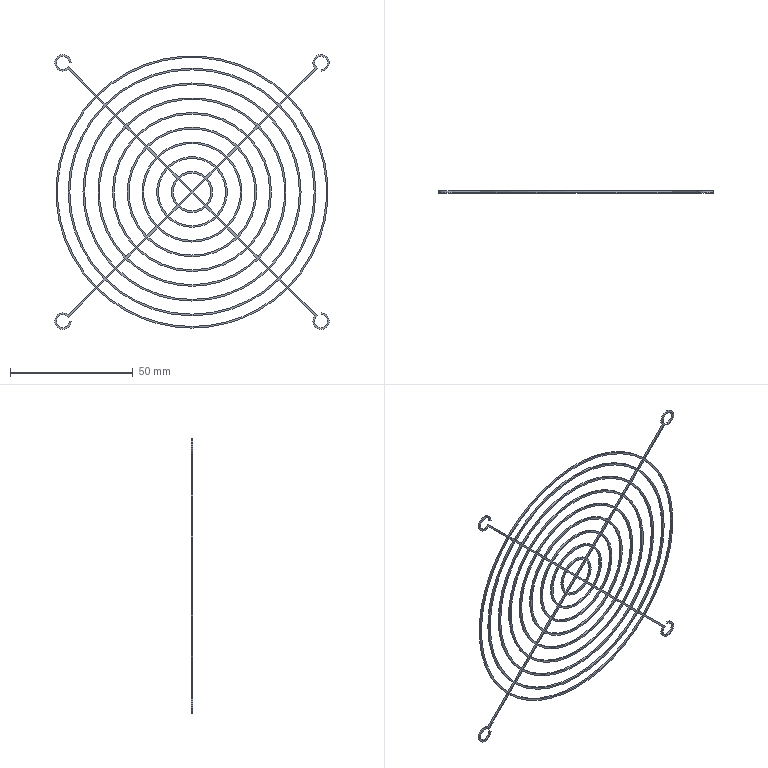Part | SolidWorks | features BaseBody 1 | 1 solid | 194 faces | box 111.7 x 0.7 x 111.7 mm | volume 1043 mm3 | cylinder 108 | plane 86 | commonest cylinder face diameters 5.3 x9 6.7 x9 15.3 x5 16.7 x5 27.3 x5 28.7 x5